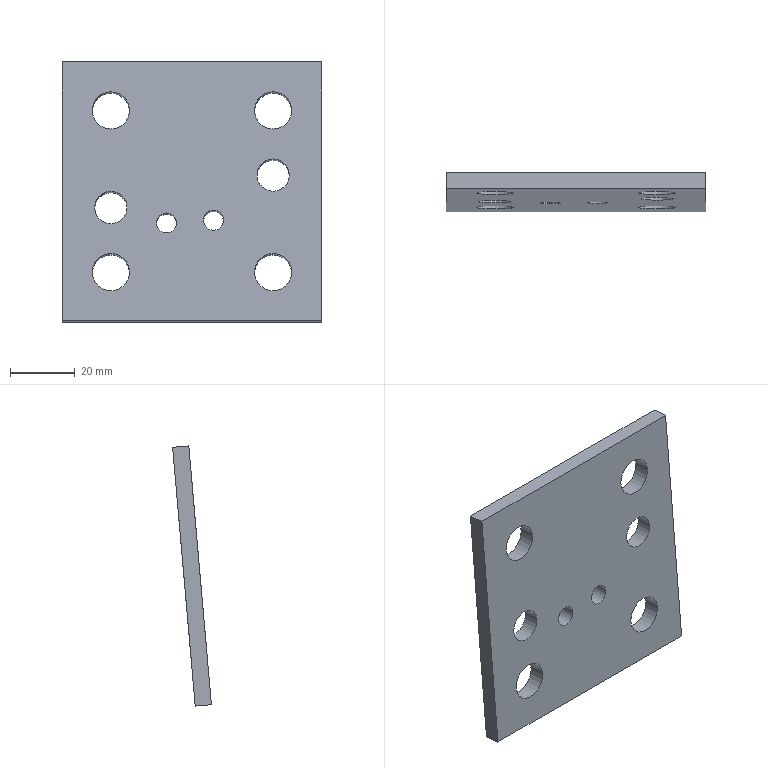Part | NX | features solid 2 | 1 solid | 14 faces | box 80 x 11.953 x 80.131 mm | volume 28835 mm3 | cylinder 8 | plane 6 | commonest cylinder face diameters 11.5 x4 6.2 x2 10 x2
STEP:
#1=CARTESIAN_POINT('',(-228.366,-148.127,-27.194));
#2=VERTEX_POINT('',#1);
#3=CARTESIAN_POINT('',(-228.366,-147.857,-24.106));
#4=DIRECTION('',(0.,-0.9962,0.08716));
#5=DIRECTION('',(0.,-0.08716,-0.9962));
#6=AXIS2_PLACEMENT_3D('',#3,#4,#5);
#7=CIRCLE('',#6,3.1);
#8=EDGE_CURVE('',#2,#2,#7,.F.);
#9=ORIENTED_EDGE('',*,*,#8,.T.);
#10=EDGE_LOOP('',(#9));
#11=FACE_BOUND('',#10,.T.);
#12=CARTESIAN_POINT('',(-242.835,-148.201,-28.036));
#13=VERTEX_POINT('',#12);
#14=CARTESIAN_POINT('',(-242.835,-147.931,-24.947));
#15=DIRECTION('',(0.,-0.9962,0.08716));
#16=DIRECTION('',(0.,-0.08716,-0.9962));
#17=AXIS2_PLACEMENT_3D('',#14,#15,#16);
#18=CIRCLE('',#17,3.1);
#19=EDGE_CURVE('',#13,#13,#18,.F.);
#20=ORIENTED_EDGE('',*,*,#19,.T.);
#21=EDGE_LOOP('',(#20));
#22=FACE_BOUND('',#21,.T.);
#23=CARTESIAN_POINT('',(-210.,-145.401,3.964));
#24=VERTEX_POINT('',#23);
#25=CARTESIAN_POINT('',(-210.,-144.9,9.692));
#26=DIRECTION('',(0.,-0.9962,0.08716));
#27=DIRECTION('',(0.,-0.08716,-0.9962));
#28=AXIS2_PLACEMENT_3D('',#25,#26,#27);
#29=CIRCLE('',#28,5.75);
#30=EDGE_CURVE('',#24,#24,#29,.F.);
#31=ORIENTED_EDGE('',*,*,#30,.T.);
#32=EDGE_LOOP('',(#31));
#33=FACE_BOUND('',#32,.T.);
#34=CARTESIAN_POINT('',(-210.,-147.079,-15.213));
#35=VERTEX_POINT('',#34);
#36=CARTESIAN_POINT('',(-210.,-146.643,-10.232));
#37=DIRECTION('',(0.,-0.9962,0.08716));
#38=DIRECTION('',(0.,-0.08716,-0.9962));
#39=AXIS2_PLACEMENT_3D('',#36,#37,#38);
#40=CIRCLE('',#39,5.);
#41=EDGE_CURVE('',#35,#35,#40,.F.);
#42=ORIENTED_EDGE('',*,*,#41,.T.);
#43=EDGE_LOOP('',(#42));
#44=FACE_BOUND('',#43,.T.);
#45=CARTESIAN_POINT('',(-260.,-145.401,3.964));
#46=VERTEX_POINT('',#45);
#47=CARTESIAN_POINT('',(-260.,-144.9,9.692));
#48=DIRECTION('',(0.,-0.9962,0.08716));
#49=DIRECTION('',(0.,-0.08716,-0.9962));
#50=AXIS2_PLACEMENT_3D('',#47,#48,#49);
#51=CIRCLE('',#50,5.75);
#52=EDGE_CURVE('',#46,#46,#51,.T.);
#53=ORIENTED_EDGE('',*,*,#52,.F.);
#54=EDGE_LOOP('',(#53));
#55=FACE_BOUND('',#54,.T.);
#56=CARTESIAN_POINT('',(-195.,-143.593,24.635));
#57=VERTEX_POINT('',#56);
#58=CARTESIAN_POINT('',(-275.,-143.593,24.635));
#59=VERTEX_POINT('',#58);
#60=CARTESIAN_POINT('',(-195.,-143.593,24.635));
#61=DIRECTION('',(-1.,0.,0.));
#62=VECTOR('',#61,1000.);
#63=LINE('',#60,#62);
#64=EDGE_CURVE('',#57,#59,#63,.T.);
#65=ORIENTED_EDGE('',*,*,#64,.T.);
#66=CARTESIAN_POINT('',(-275.,-150.565,-55.061));
#67=VERTEX_POINT('',#66);
#68=CARTESIAN_POINT('',(-275.,-143.07,30.61));
#69=DIRECTION('',(0.,-0.08716,-0.9962));
#70=VECTOR('',#69,1000.);
#71=LINE('',#68,#70);
#72=EDGE_CURVE('',#67,#59,#71,.F.);
#73=ORIENTED_EDGE('',*,*,#72,.F.);
#74=CARTESIAN_POINT('',(-195.,-150.565,-55.061));
#75=VERTEX_POINT('',#74);
#76=CARTESIAN_POINT('',(-195.,-150.565,-55.061));
#77=DIRECTION('',(1.,0.,0.));
#78=VECTOR('',#77,1000.);
#79=LINE('',#76,#78);
#80=EDGE_CURVE('',#67,#75,#79,.T.);
#81=ORIENTED_EDGE('',*,*,#80,.T.);
#82=CARTESIAN_POINT('',(-195.,-147.646,-21.689));
#83=DIRECTION('',(0.,-0.08716,-0.9962));
#84=VECTOR('',#83,1000.);
#85=LINE('',#82,#84);
#86=EDGE_CURVE('',#57,#75,#85,.T.);
#87=ORIENTED_EDGE('',*,*,#86,.F.);
#88=EDGE_LOOP('',(#65,#73,#81,#87));
#89=FACE_BOUND('',#88,.T.);
#90=CARTESIAN_POINT('',(-260.,-147.951,-25.175));
#91=VERTEX_POINT('',#90);
#92=CARTESIAN_POINT('',(-260.,-147.515,-20.194));
#93=DIRECTION('',(0.,-0.9962,0.08716));
#94=DIRECTION('',(0.,-0.08716,-0.9962));
#95=AXIS2_PLACEMENT_3D('',#92,#93,#94);
#96=CIRCLE('',#95,5.);
#97=EDGE_CURVE('',#91,#91,#96,.F.);
#98=ORIENTED_EDGE('',*,*,#97,.T.);
#99=EDGE_LOOP('',(#98));
#100=FACE_BOUND('',#99,.T.);
#101=CARTESIAN_POINT('',(-260.,-149.759,-45.846));
#102=VERTEX_POINT('',#101);
#103=CARTESIAN_POINT('',(-260.,-149.258,-40.118));
#104=DIRECTION('',(0.,-0.9962,0.08716));
#105=DIRECTION('',(0.,-0.08716,-0.9962));
#106=AXIS2_PLACEMENT_3D('',#103,#104,#105);
#107=CIRCLE('',#106,5.75);
#108=EDGE_CURVE('',#102,#102,#107,.F.);
#109=ORIENTED_EDGE('',*,*,#108,.T.);
#110=EDGE_LOOP('',(#109));
#111=FACE_BOUND('',#110,.T.);
#112=CARTESIAN_POINT('',(-210.,-149.759,-45.846));
#113=VERTEX_POINT('',#112);
#114=CARTESIAN_POINT('',(-210.,-149.258,-40.118));
#115=DIRECTION('',(0.,-0.9962,0.08716));
#116=DIRECTION('',(0.,-0.08716,-0.9962));
#117=AXIS2_PLACEMENT_3D('',#114,#115,#116);
#118=CIRCLE('',#117,5.75);
#119=EDGE_CURVE('',#113,#113,#118,.T.);
#120=ORIENTED_EDGE('',*,*,#119,.F.);
#121=EDGE_LOOP('',(#120));
#122=FACE_BOUND('',#121,.T.);
#123=CARTESIAN_POINT('',(-195.,-143.07,30.61));
#124=DIRECTION('',(0.,-0.9962,0.08716));
#125=DIRECTION('',(-1.,0.,0.));
#126=AXIS2_PLACEMENT_3D('',#123,#124,#125);
#127=PLANE('',#126);
#128=ADVANCED_FACE('',(#11,#22,#33,#44,#55,#89,#100,#111,#122),#127,.T.);
#129=CARTESIAN_POINT('',(-228.366,-143.146,-27.63));
#130=VERTEX_POINT('',#129);
#131=CARTESIAN_POINT('',(-228.366,-142.876,-24.542));
#132=DIRECTION('',(0.,-0.9962,0.08716));
#133=DIRECTION('',(0.,-0.08716,-0.9962));
#134=AXIS2_PLACEMENT_3D('',#131,#132,#133);
#135=CIRCLE('',#134,3.1);
#136=EDGE_CURVE('',#130,#130,#135,.F.);
#137=ORIENTED_EDGE('',*,*,#136,.F.);
#138=EDGE_LOOP('',(#137));
#139=FACE_BOUND('',#138,.T.);
#140=CARTESIAN_POINT('',(-242.835,-143.22,-28.471));
#141=VERTEX_POINT('',#140);
#142=CARTESIAN_POINT('',(-242.835,-142.95,-25.383));
#143=DIRECTION('',(0.,-0.9962,0.08716));
#144=DIRECTION('',(0.,-0.08716,-0.9962));
#145=AXIS2_PLACEMENT_3D('',#142,#143,#144);
#146=CIRCLE('',#145,3.1);
#147=EDGE_CURVE('',#141,#141,#146,.F.);
#148=ORIENTED_EDGE('',*,*,#147,.F.);
#149=EDGE_LOOP('',(#148));
#150=FACE_BOUND('',#149,.T.);
#151=CARTESIAN_POINT('',(-210.,-140.42,3.528));
#152=VERTEX_POINT('',#151);
#153=CARTESIAN_POINT('',(-210.,-139.919,9.256));
#154=DIRECTION('',(0.,-0.9962,0.08716));
#155=DIRECTION('',(0.,-0.08716,-0.9962));
#156=AXIS2_PLACEMENT_3D('',#153,#154,#155);
#157=CIRCLE('',#156,5.75);
#158=EDGE_CURVE('',#152,#152,#157,.F.);
#159=ORIENTED_EDGE('',*,*,#158,.F.);
#160=EDGE_LOOP('',(#159));
#161=FACE_BOUND('',#160,.T.);
#162=CARTESIAN_POINT('',(-210.,-142.098,-15.649));
#163=VERTEX_POINT('',#162);
#164=CARTESIAN_POINT('',(-210.,-141.662,-10.668));
#165=DIRECTION('',(0.,-0.9962,0.08716));
#166=DIRECTION('',(0.,-0.08716,-0.9962));
#167=AXIS2_PLACEMENT_3D('',#164,#165,#166);
#168=CIRCLE('',#167,5.);
#169=EDGE_CURVE('',#163,#163,#168,.F.);
#170=ORIENTED_EDGE('',*,*,#169,.F.);
#171=EDGE_LOOP('',(#170));
#172=FACE_BOUND('',#171,.T.);
#173=CARTESIAN_POINT('',(-260.,-140.42,3.528));
#174=VERTEX_POINT('',#173);
#175=CARTESIAN_POINT('',(-260.,-139.919,9.256));
#176=DIRECTION('',(0.,-0.9962,0.08716));
#177=DIRECTION('',(0.,-0.08716,-0.9962));
#178=AXIS2_PLACEMENT_3D('',#175,#176,#177);
#179=CIRCLE('',#178,5.75);
#180=EDGE_CURVE('',#174,#174,#179,.T.);
#181=ORIENTED_EDGE('',*,*,#180,.T.);
#182=EDGE_LOOP('',(#181));
#183=FACE_BOUND('',#182,.T.);
#184=CARTESIAN_POINT('',(-195.,-138.612,24.199));
#185=VERTEX_POINT('',#184);
#186=CARTESIAN_POINT('',(-275.,-138.612,24.199));
#187=VERTEX_POINT('',#186);
#188=CARTESIAN_POINT('',(-195.,-138.612,24.199));
#189=DIRECTION('',(-1.,0.,0.));
#190=VECTOR('',#189,1000.);
#191=LINE('',#188,#190);
#192=EDGE_CURVE('',#185,#187,#191,.T.);
#193=ORIENTED_EDGE('',*,*,#192,.F.);
#194=CARTESIAN_POINT('',(-195.,-145.584,-55.497));
#195=VERTEX_POINT('',#194);
#196=CARTESIAN_POINT('',(-195.,-142.665,-22.124));
#197=DIRECTION('',(0.,-0.08716,-0.9962));
#198=VECTOR('',#197,1000.);
#199=LINE('',#196,#198);
#200=EDGE_CURVE('',#185,#195,#199,.T.);
#201=ORIENTED_EDGE('',*,*,#200,.T.);
#202=CARTESIAN_POINT('',(-275.,-145.584,-55.497));
#203=VERTEX_POINT('',#202);
#204=CARTESIAN_POINT('',(-195.,-145.584,-55.497));
#205=DIRECTION('',(-1.,0.,0.));
#206=VECTOR('',#205,1000.);
#207=LINE('',#204,#206);
#208=EDGE_CURVE('',#203,#195,#207,.F.);
#209=ORIENTED_EDGE('',*,*,#208,.F.);
#210=CARTESIAN_POINT('',(-275.,-138.089,30.174));
#211=DIRECTION('',(0.,-0.08716,-0.9962));
#212=VECTOR('',#211,1000.);
#213=LINE('',#210,#212);
#214=EDGE_CURVE('',#203,#187,#213,.F.);
#215=ORIENTED_EDGE('',*,*,#214,.T.);
#216=EDGE_LOOP('',(#193,#201,#209,#215));
#217=FACE_BOUND('',#216,.T.);
#218=CARTESIAN_POINT('',(-260.,-142.97,-25.611));
#219=VERTEX_POINT('',#218);
#220=CARTESIAN_POINT('',(-260.,-142.534,-20.63));
#221=DIRECTION('',(0.,-0.9962,0.08716));
#222=DIRECTION('',(0.,-0.08716,-0.9962));
#223=AXIS2_PLACEMENT_3D('',#220,#221,#222);
#224=CIRCLE('',#223,5.);
#225=EDGE_CURVE('',#219,#219,#224,.F.);
#226=ORIENTED_EDGE('',*,*,#225,.F.);
#227=EDGE_LOOP('',(#226));
#228=FACE_BOUND('',#227,.T.);
#229=CARTESIAN_POINT('',(-260.,-144.778,-46.282));
#230=VERTEX_POINT('',#229);
#231=CARTESIAN_POINT('',(-260.,-144.277,-40.554));
#232=DIRECTION('',(0.,-0.9962,0.08716));
#233=DIRECTION('',(0.,-0.08716,-0.9962));
#234=AXIS2_PLACEMENT_3D('',#231,#232,#233);
#235=CIRCLE('',#234,5.75);
#236=EDGE_CURVE('',#230,#230,#235,.F.);
#237=ORIENTED_EDGE('',*,*,#236,.F.);
#238=EDGE_LOOP('',(#237));
#239=FACE_BOUND('',#238,.T.);
#240=CARTESIAN_POINT('',(-210.,-144.778,-46.282));
#241=VERTEX_POINT('',#240);
#242=CARTESIAN_POINT('',(-210.,-144.277,-40.554));
#243=DIRECTION('',(0.,-0.9962,0.08716));
#244=DIRECTION('',(0.,-0.08716,-0.9962));
#245=AXIS2_PLACEMENT_3D('',#242,#243,#244);
#246=CIRCLE('',#245,5.75);
#247=EDGE_CURVE('',#241,#241,#246,.T.);
#248=ORIENTED_EDGE('',*,*,#247,.T.);
#249=EDGE_LOOP('',(#248));
#250=FACE_BOUND('',#249,.T.);
#251=CARTESIAN_POINT('',(-195.,-138.089,30.174));
#252=DIRECTION('',(0.,-0.9962,0.08716));
#253=DIRECTION('',(-1.,0.,0.));
#254=AXIS2_PLACEMENT_3D('',#251,#252,#253);
#255=PLANE('',#254);
#256=ADVANCED_FACE('',(#139,#150,#161,#172,#183,#217,#228,#239,#250),#255,.F.);
#257=ORIENTED_EDGE('',*,*,#192,.T.);
#258=CARTESIAN_POINT('',(-275.,-143.593,24.635));
#259=DIRECTION('',(0.,0.9962,-0.08716));
#260=VECTOR('',#259,1000.);
#261=LINE('',#258,#260);
#262=EDGE_CURVE('',#59,#187,#261,.T.);
#263=ORIENTED_EDGE('',*,*,#262,.F.);
#264=ORIENTED_EDGE('',*,*,#64,.F.);
#265=CARTESIAN_POINT('',(-195.,-143.593,24.635));
#266=DIRECTION('',(0.,0.9962,-0.08716));
#267=VECTOR('',#266,1000.);
#268=LINE('',#265,#267);
#269=EDGE_CURVE('',#57,#185,#268,.T.);
#270=ORIENTED_EDGE('',*,*,#269,.T.);
#271=EDGE_LOOP('',(#257,#263,#264,#270));
#272=FACE_BOUND('',#271,.T.);
#273=CARTESIAN_POINT('',(-195.,-143.593,24.635));
#274=DIRECTION('',(0.,-0.08716,-0.9962));
#275=DIRECTION('',(0.,0.9962,-0.08716));
#276=AXIS2_PLACEMENT_3D('',#273,#274,#275);
#277=PLANE('',#276);
#278=ADVANCED_FACE('',(#272),#277,.F.);
#279=ORIENTED_EDGE('',*,*,#200,.F.);
#280=ORIENTED_EDGE('',*,*,#269,.F.);
#281=ORIENTED_EDGE('',*,*,#86,.T.);
#282=CARTESIAN_POINT('',(-195.,-150.565,-55.061));
#283=DIRECTION('',(0.,-0.9962,0.08716));
#284=VECTOR('',#283,1000.);
#285=LINE('',#282,#284);
#286=EDGE_CURVE('',#75,#195,#285,.F.);
#287=ORIENTED_EDGE('',*,*,#286,.T.);
#288=EDGE_LOOP('',(#279,#280,#281,#287));
#289=FACE_BOUND('',#288,.T.);
#290=CARTESIAN_POINT('',(-195.,-147.646,-21.689));
#291=DIRECTION('',(1.,0.,0.));
#292=DIRECTION('',(0.,0.,-1.));
#293=AXIS2_PLACEMENT_3D('',#290,#291,#292);
#294=PLANE('',#293);
#295=ADVANCED_FACE('',(#289),#294,.T.);
#296=ORIENTED_EDGE('',*,*,#208,.T.);
#297=ORIENTED_EDGE('',*,*,#286,.F.);
#298=ORIENTED_EDGE('',*,*,#80,.F.);
#299=CARTESIAN_POINT('',(-275.,-150.565,-55.061));
#300=DIRECTION('',(0.,0.9962,-0.08716));
#301=VECTOR('',#300,1000.);
#302=LINE('',#299,#301);
#303=EDGE_CURVE('',#67,#203,#302,.T.);
#304=ORIENTED_EDGE('',*,*,#303,.T.);
#305=EDGE_LOOP('',(#296,#297,#298,#304));
#306=FACE_BOUND('',#305,.T.);
#307=CARTESIAN_POINT('',(-195.,-150.565,-55.061));
#308=DIRECTION('',(0.,-0.08716,-0.9962));
#309=DIRECTION('',(0.,0.9962,-0.08716));
#310=AXIS2_PLACEMENT_3D('',#307,#308,#309);
#311=PLANE('',#310);
#312=ADVANCED_FACE('',(#306),#311,.T.);
#313=ORIENTED_EDGE('',*,*,#214,.F.);
#314=ORIENTED_EDGE('',*,*,#303,.F.);
#315=ORIENTED_EDGE('',*,*,#72,.T.);
#316=ORIENTED_EDGE('',*,*,#262,.T.);
#317=EDGE_LOOP('',(#313,#314,#315,#316));
#318=FACE_BOUND('',#317,.T.);
#319=CARTESIAN_POINT('',(-275.,-143.07,30.61));
#320=DIRECTION('',(-1.,0.,0.));
#321=DIRECTION('',(0.,0.,1.));
#322=AXIS2_PLACEMENT_3D('',#319,#320,#321);
#323=PLANE('',#322);
#324=ADVANCED_FACE('',(#318),#323,.T.);
#325=ORIENTED_EDGE('',*,*,#180,.F.);
#326=EDGE_LOOP('',(#325));
#327=FACE_BOUND('',#326,.T.);
#328=ORIENTED_EDGE('',*,*,#52,.T.);
#329=EDGE_LOOP('',(#328));
#330=FACE_BOUND('',#329,.T.);
#331=CARTESIAN_POINT('',(-260.,-115.014,7.077));
#332=DIRECTION('',(0.,-0.9962,0.08716));
#333=DIRECTION('',(1.,0.,0.));
#334=AXIS2_PLACEMENT_3D('',#331,#332,#333);
#335=CYLINDRICAL_SURFACE('',#334,5.75);
#336=ADVANCED_FACE('',(#327,#330),#335,.F.);
#337=ORIENTED_EDGE('',*,*,#225,.T.);
#338=EDGE_LOOP('',(#337));
#339=FACE_BOUND('',#338,.T.);
#340=ORIENTED_EDGE('',*,*,#97,.F.);
#341=EDGE_LOOP('',(#340));
#342=FACE_BOUND('',#341,.T.);
#343=CARTESIAN_POINT('',(-260.,-117.629,-22.809));
#344=DIRECTION('',(0.,-0.9962,0.08716));
#345=DIRECTION('',(1.,0.,0.));
#346=AXIS2_PLACEMENT_3D('',#343,#344,#345);
#347=CYLINDRICAL_SURFACE('',#346,5.);
#348=ADVANCED_FACE('',(#339,#342),#347,.F.);
#349=ORIENTED_EDGE('',*,*,#236,.T.);
#350=EDGE_LOOP('',(#349));
#351=FACE_BOUND('',#350,.T.);
#352=ORIENTED_EDGE('',*,*,#108,.F.);
#353=EDGE_LOOP('',(#352));
#354=FACE_BOUND('',#353,.T.);
#355=CARTESIAN_POINT('',(-260.,-119.372,-42.733));
#356=DIRECTION('',(0.,-0.9962,0.08716));
#357=DIRECTION('',(1.,0.,0.));
#358=AXIS2_PLACEMENT_3D('',#355,#356,#357);
#359=CYLINDRICAL_SURFACE('',#358,5.75);
#360=ADVANCED_FACE('',(#351,#354),#359,.F.);
#361=ORIENTED_EDGE('',*,*,#247,.F.);
#362=EDGE_LOOP('',(#361));
#363=FACE_BOUND('',#362,.T.);
#364=ORIENTED_EDGE('',*,*,#119,.T.);
#365=EDGE_LOOP('',(#364));
#366=FACE_BOUND('',#365,.T.);
#367=CARTESIAN_POINT('',(-210.,-119.372,-42.733));
#368=DIRECTION('',(0.,-0.9962,0.08716));
#369=DIRECTION('',(1.,0.,0.));
#370=AXIS2_PLACEMENT_3D('',#367,#368,#369);
#371=CYLINDRICAL_SURFACE('',#370,5.75);
#372=ADVANCED_FACE('',(#363,#366),#371,.F.);
#373=ORIENTED_EDGE('',*,*,#169,.T.);
#374=EDGE_LOOP('',(#373));
#375=FACE_BOUND('',#374,.T.);
#376=ORIENTED_EDGE('',*,*,#41,.F.);
#377=EDGE_LOOP('',(#376));
#378=FACE_BOUND('',#377,.T.);
#379=CARTESIAN_POINT('',(-210.,-116.757,-12.847));
#380=DIRECTION('',(0.,-0.9962,0.08716));
#381=DIRECTION('',(1.,0.,0.));
#382=AXIS2_PLACEMENT_3D('',#379,#380,#381);
#383=CYLINDRICAL_SURFACE('',#382,5.);
#384=ADVANCED_FACE('',(#375,#378),#383,.F.);
#385=ORIENTED_EDGE('',*,*,#158,.T.);
#386=EDGE_LOOP('',(#385));
#387=FACE_BOUND('',#386,.T.);
#388=ORIENTED_EDGE('',*,*,#30,.F.);
#389=EDGE_LOOP('',(#388));
#390=FACE_BOUND('',#389,.T.);
#391=CARTESIAN_POINT('',(-210.,-115.014,7.077));
#392=DIRECTION('',(0.,-0.9962,0.08716));
#393=DIRECTION('',(1.,0.,0.));
#394=AXIS2_PLACEMENT_3D('',#391,#392,#393);
#395=CYLINDRICAL_SURFACE('',#394,5.75);
#396=ADVANCED_FACE('',(#387,#390),#395,.F.);
#397=ORIENTED_EDGE('',*,*,#147,.T.);
#398=EDGE_LOOP('',(#397));
#399=FACE_BOUND('',#398,.T.);
#400=ORIENTED_EDGE('',*,*,#19,.F.);
#401=EDGE_LOOP('',(#400));
#402=FACE_BOUND('',#401,.T.);
#403=CARTESIAN_POINT('',(-242.835,-43.33,-34.099));
#404=DIRECTION('',(0.,-0.9962,0.08716));
#405=DIRECTION('',(1.,0.,0.));
#406=AXIS2_PLACEMENT_3D('',#403,#404,#405);
#407=CYLINDRICAL_SURFACE('',#406,3.1);
#408=ADVANCED_FACE('',(#399,#402),#407,.F.);
#409=ORIENTED_EDGE('',*,*,#136,.T.);
#410=EDGE_LOOP('',(#409));
#411=FACE_BOUND('',#410,.T.);
#412=ORIENTED_EDGE('',*,*,#8,.F.);
#413=EDGE_LOOP('',(#412));
#414=FACE_BOUND('',#413,.T.);
#415=CARTESIAN_POINT('',(-228.366,-43.257,-33.257));
#416=DIRECTION('',(0.,-0.9962,0.08716));
#417=DIRECTION('',(1.,0.,0.));
#418=AXIS2_PLACEMENT_3D('',#415,#416,#417);
#419=CYLINDRICAL_SURFACE('',#418,3.1);
#420=ADVANCED_FACE('',(#411,#414),#419,.F.);
#421=CLOSED_SHELL('',(#128,#256,#278,#295,#312,#324,#336,#348,#360,#372,#384,#396,#408,#420));
#422=MANIFOLD_SOLID_BREP('',#421);
#423=(LENGTH_UNIT()NAMED_UNIT(*)SI_UNIT(.MILLI.,.METRE.));
#424=UNCERTAINTY_MEASURE_WITH_UNIT(LENGTH_MEASURE(0.00001),#423,'','');
#425=(NAMED_UNIT(*)PLANE_ANGLE_UNIT()SI_UNIT($,.RADIAN.));
#426=(NAMED_UNIT(*)SI_UNIT($,.STERADIAN.)SOLID_ANGLE_UNIT());
#427=(GEOMETRIC_REPRESENTATION_CONTEXT(3)GLOBAL_UNCERTAINTY_ASSIGNED_CONTEXT((#424))GLOBAL_UNIT_ASSIGNED_CONTEXT((#423,#425,#426))REPRESENTATION_CONTEXT('',''));
#428=ADVANCED_BREP_SHAPE_REPRESENTATION('',(#422),#427);